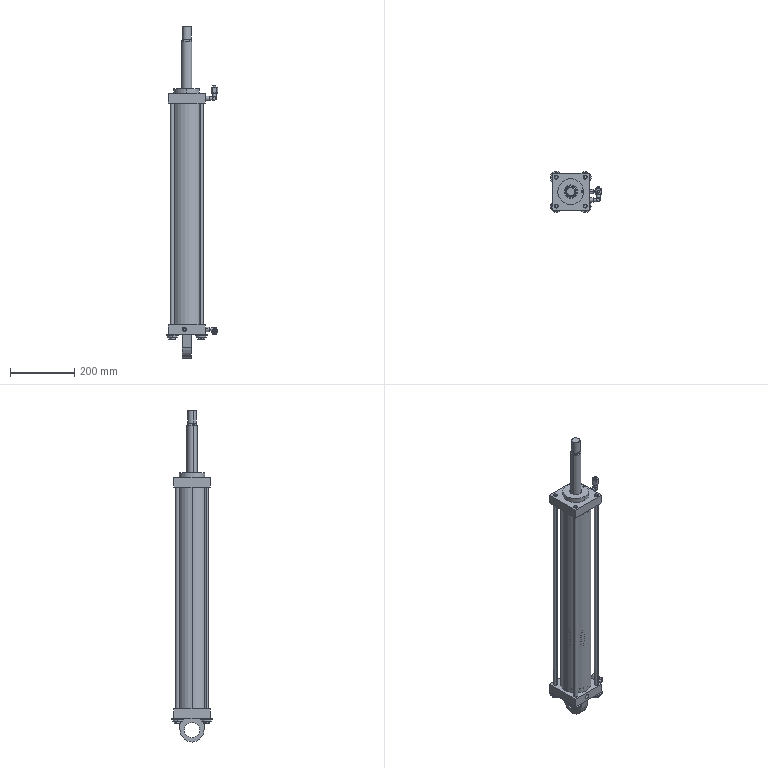Part | SolidWorks | features ReferencePattern 9, LocalCirPattern 1 | 19 solids | 585 faces | box 159.892 x 127 x 1033 mm | volume 2737892 mm3 | cylinder 254 | plane 190 | cone 127 | torus 10 | sphere 2 | spline 2 | commonest cylinder face diameters 3.2 x32 6 x25 90 x18 12.5 x16 4 x12 20.2 x12